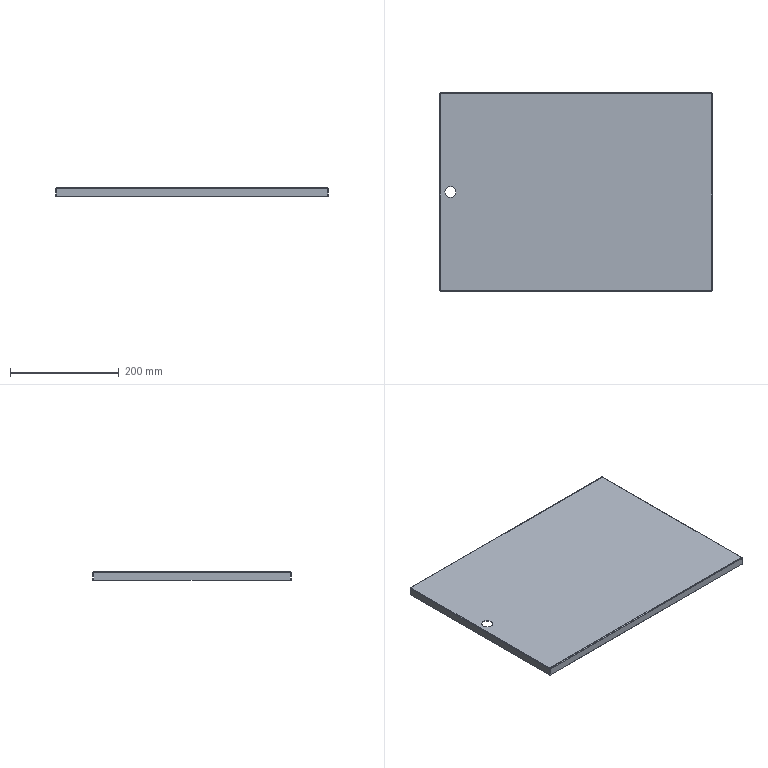Part | STEP file | x77-05303 | 1 solid | 40 faces | box 502 x 365 x 15 mm | volume 206076 mm3 | plane 22 | cylinder 10 | spline 8 | commonest cylinder face diameters 1.473 x4 3.473 x4 20 x2